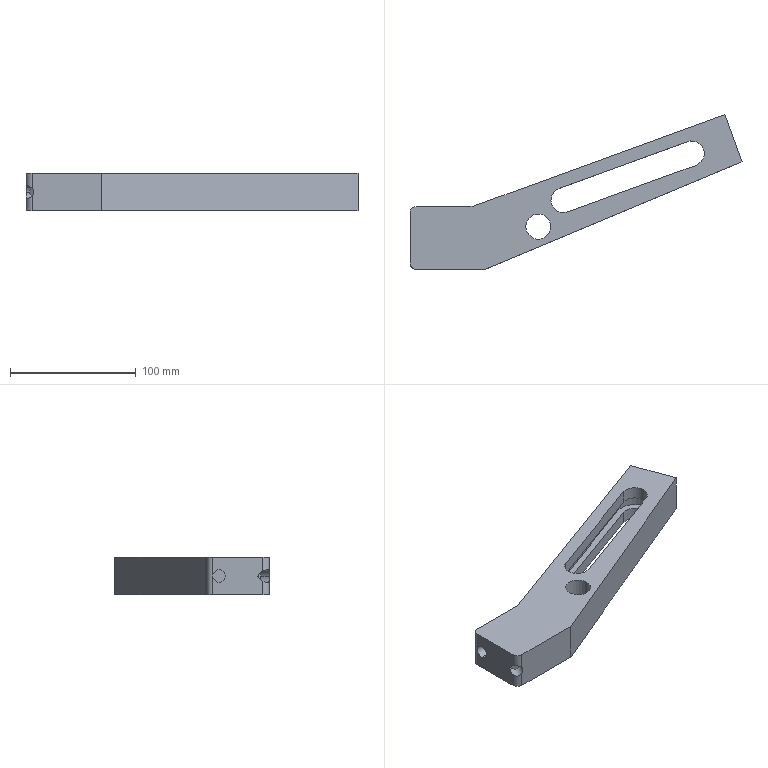Part | SolidWorks | features ICE 8, Fillet 2, Extrusion 1 | 1 solid | 37 faces | box 264.316 x 123.025 x 30 mm | volume 276042 mm3 | cylinder 19 | plane 18 | commonest cylinder face diameters 20 x9 10 x7 30 x3
STEP:
#1=CARTESIAN_POINT('',(239.287,92.152,-5.));
#2=VERTEX_POINT('',#1);
#3=CARTESIAN_POINT('',(219.156,106.247,-5.));
#4=VERTEX_POINT('',#3);
#5=CARTESIAN_POINT('',(224.287,92.152,-5.));
#6=DIRECTION('',(0.,0.,1.));
#7=DIRECTION('',(1.,0.,0.));
#8=AXIS2_PLACEMENT_3D('',#5,#6,#7);
#9=CIRCLE('',#8,15.);
#10=EDGE_CURVE('',#2,#4,#9,.T.);
#11=ORIENTED_EDGE('',*,*,#10,.F.);
#12=CARTESIAN_POINT('',(239.287,92.152,5.));
#13=VERTEX_POINT('',#12);
#14=CARTESIAN_POINT('',(239.287,92.152,-5.));
#15=DIRECTION('',(0.,0.,1.));
#16=VECTOR('',#15,1000.);
#17=LINE('',#14,#16);
#18=EDGE_CURVE('',#2,#13,#17,.T.);
#19=ORIENTED_EDGE('',*,*,#18,.T.);
#20=CARTESIAN_POINT('',(219.156,106.247,5.));
#21=VERTEX_POINT('',#20);
#22=CARTESIAN_POINT('',(224.287,92.152,5.));
#23=DIRECTION('',(0.,0.,1.));
#24=DIRECTION('',(1.,0.,0.));
#25=AXIS2_PLACEMENT_3D('',#22,#23,#24);
#26=CIRCLE('',#25,15.);
#27=EDGE_CURVE('',#13,#21,#26,.T.);
#28=ORIENTED_EDGE('',*,*,#27,.T.);
#29=CARTESIAN_POINT('',(219.156,106.247,-5.));
#30=DIRECTION('',(0.,0.,1.));
#31=VECTOR('',#30,1000.);
#32=LINE('',#29,#31);
#33=EDGE_CURVE('',#4,#21,#32,.T.);
#34=ORIENTED_EDGE('',*,*,#33,.F.);
#35=EDGE_LOOP('',(#11,#19,#28,#34));
#36=FACE_OUTER_BOUND('',#35,.T.);
#37=CARTESIAN_POINT('',(224.287,92.152,-5.));
#38=DIRECTION('',(0.,0.,1.));
#39=DIRECTION('',(1.,0.,0.));
#40=AXIS2_PLACEMENT_3D('',#37,#38,#39);
#41=CYLINDRICAL_SURFACE('',#40,15.);
#42=ADVANCED_FACE('',(#36),#41,.F.);
#43=CARTESIAN_POINT('',(112.167,33.891,-15.));
#44=VERTEX_POINT('',#43);
#45=CARTESIAN_POINT('',(92.167,33.891,-15.));
#46=VERTEX_POINT('',#45);
#47=CARTESIAN_POINT('',(102.167,33.891,-15.));
#48=DIRECTION('',(0.,0.,-1.));
#49=DIRECTION('',(-1.,0.,0.));
#50=AXIS2_PLACEMENT_3D('',#47,#48,#49);
#51=CIRCLE('',#50,10.);
#52=EDGE_CURVE('',#44,#46,#51,.T.);
#53=ORIENTED_EDGE('',*,*,#52,.T.);
#54=CARTESIAN_POINT('',(92.167,33.891,15.));
#55=VERTEX_POINT('',#54);
#56=CARTESIAN_POINT('',(92.167,33.891,-65.));
#57=DIRECTION('',(0.,0.,1.));
#58=VECTOR('',#57,1000.);
#59=LINE('',#56,#58);
#60=EDGE_CURVE('',#46,#55,#59,.T.);
#61=ORIENTED_EDGE('',*,*,#60,.T.);
#62=CARTESIAN_POINT('',(112.167,33.891,15.));
#63=VERTEX_POINT('',#62);
#64=CARTESIAN_POINT('',(102.167,33.891,15.));
#65=DIRECTION('',(0.,0.,1.));
#66=DIRECTION('',(1.,0.,0.));
#67=AXIS2_PLACEMENT_3D('',#64,#65,#66);
#68=CIRCLE('',#67,10.);
#69=EDGE_CURVE('',#55,#63,#68,.T.);
#70=ORIENTED_EDGE('',*,*,#69,.T.);
#71=CARTESIAN_POINT('',(112.167,33.891,-65.));
#72=DIRECTION('',(0.,0.,1.));
#73=VECTOR('',#72,1000.);
#74=LINE('',#71,#73);
#75=EDGE_CURVE('',#44,#63,#74,.T.);
#76=ORIENTED_EDGE('',*,*,#75,.F.);
#77=EDGE_LOOP('',(#53,#61,#70,#76));
#78=FACE_OUTER_BOUND('',#77,.T.);
#79=CARTESIAN_POINT('',(102.167,33.891,-65.));
#80=DIRECTION('',(0.,0.,1.));
#81=DIRECTION('',(1.,0.,0.));
#82=AXIS2_PLACEMENT_3D('',#79,#80,#81);
#83=CYLINDRICAL_SURFACE('',#82,10.);
#84=ADVANCED_FACE('',(#78),#83,.F.);
#85=CARTESIAN_POINT('',(10.,40.,-5.));
#86=VERTEX_POINT('',#85);
#87=CARTESIAN_POINT('',(10.,40.,5.));
#88=VERTEX_POINT('',#87);
#89=CARTESIAN_POINT('',(10.,40.,0.));
#90=DIRECTION('',(-1.,0.,0.));
#91=DIRECTION('',(0.,0.,1.));
#92=AXIS2_PLACEMENT_3D('',#89,#90,#91);
#93=CIRCLE('',#92,5.);
#94=EDGE_CURVE('',#86,#88,#93,.T.);
#95=ORIENTED_EDGE('',*,*,#94,.F.);
#96=CARTESIAN_POINT('',(0.,40.,-5.));
#97=VERTEX_POINT('',#96);
#98=CARTESIAN_POINT('',(10.,40.,-5.));
#99=DIRECTION('',(-1.,0.,0.));
#100=VECTOR('',#99,1000.);
#101=LINE('',#98,#100);
#102=EDGE_CURVE('',#86,#97,#101,.T.);
#103=ORIENTED_EDGE('',*,*,#102,.T.);
#104=CARTESIAN_POINT('',(0.,40.,5.));
#105=VERTEX_POINT('',#104);
#106=CARTESIAN_POINT('',(0.,40.,0.));
#107=DIRECTION('',(-1.,0.,0.));
#108=DIRECTION('',(0.,0.,1.));
#109=AXIS2_PLACEMENT_3D('',#106,#107,#108);
#110=CIRCLE('',#109,5.);
#111=EDGE_CURVE('',#97,#105,#110,.T.);
#112=ORIENTED_EDGE('',*,*,#111,.T.);
#113=CARTESIAN_POINT('',(10.,40.,5.));
#114=DIRECTION('',(-1.,0.,0.));
#115=VECTOR('',#114,1000.);
#116=LINE('',#113,#115);
#117=EDGE_CURVE('',#88,#105,#116,.T.);
#118=ORIENTED_EDGE('',*,*,#117,.F.);
#119=EDGE_LOOP('',(#95,#103,#112,#118));
#120=FACE_OUTER_BOUND('',#119,.T.);
#121=CARTESIAN_POINT('',(10.,40.,0.));
#122=DIRECTION('',(-1.,0.,0.));
#123=DIRECTION('',(0.,0.,1.));
#124=AXIS2_PLACEMENT_3D('',#121,#122,#123);
#125=CYLINDRICAL_SURFACE('',#124,5.);
#126=ADVANCED_FACE('',(#120),#125,.F.);
#127=CARTESIAN_POINT('',(2.999,12.634,0.));
#128=VERTEX_POINT('',#127);
#129=CARTESIAN_POINT('',(11.089,6.756,0.));
#130=VERTEX_POINT('',#129);
#131=CARTESIAN_POINT('',(7.044,9.695,0.));
#132=DIRECTION('',(-0.5878,-0.809,0.));
#133=DIRECTION('',(0.809,-0.5878,0.));
#134=AXIS2_PLACEMENT_3D('',#131,#132,#133);
#135=CIRCLE('',#134,5.);
#136=EDGE_CURVE('',#128,#130,#135,.T.);
#137=ORIENTED_EDGE('',*,*,#136,.F.);
#138=CARTESIAN_POINT('',(0.,8.507,0.));
#139=VERTEX_POINT('',#138);
#140=CARTESIAN_POINT('',(2.999,12.634,0.));
#141=DIRECTION('',(-0.5878,-0.809,0.));
#142=VECTOR('',#141,1000.);
#143=LINE('',#140,#142);
#144=EDGE_CURVE('',#128,#139,#143,.T.);
#145=ORIENTED_EDGE('',*,*,#144,.T.);
#146=CARTESIAN_POINT('',(0.,5.,-4.045));
#147=VERTEX_POINT('',#146);
#148=CARTESIAN_POINT('',(0.,5.,-4.045));
#149=CARTESIAN_POINT('',(0.,7.246,-3.086));
#150=CARTESIAN_POINT('',(0.,8.507,-1.632));
#151=CARTESIAN_POINT('',(0.,8.507,0.));
#152=(BOUNDED_CURVE()B_SPLINE_CURVE(3,(#148,#149,#150,#151),.UNSPECIFIED.,.F.,.T.)B_SPLINE_CURVE_WITH_KNOTS((4,4),(2.199,3.142),.UNSPECIFIED.)CURVE()GEOMETRIC_REPRESENTATION_ITEM()RATIONAL_B_SPLINE_CURVE((1.,0.9273,0.9273,1.))REPRESENTATION_ITEM(''));
#153=EDGE_CURVE('',#147,#139,#152,.T.);
#154=ORIENTED_EDGE('',*,*,#153,.F.);
#155=CARTESIAN_POINT('',(5.,0.,-2.939));
#156=VERTEX_POINT('',#155);
#157=CARTESIAN_POINT('',(0.,5.,-4.045));
#158=CARTESIAN_POINT('',(0.,4.668,-4.187));
#159=CARTESIAN_POINT('',(0.03262,4.339,-4.325));
#160=CARTESIAN_POINT('',(0.165,3.683,-4.577));
#161=CARTESIAN_POINT('',(0.2668,3.352,-4.692));
#162=CARTESIAN_POINT('',(0.4713,2.874,-4.828));
#163=CARTESIAN_POINT('',(0.5481,2.717,-4.868));
#164=CARTESIAN_POINT('',(0.7198,2.409,-4.933));
#165=CARTESIAN_POINT('',(0.8156,2.257,-4.958));
#166=CARTESIAN_POINT('',(1.127,1.817,-5.009));
#167=CARTESIAN_POINT('',(1.363,1.55,-5.009));
#168=CARTESIAN_POINT('',(1.758,1.189,-4.951));
#169=CARTESIAN_POINT('',(1.898,1.075,-4.921));
#170=CARTESIAN_POINT('',(2.181,0.8669,-4.843));
#171=CARTESIAN_POINT('',(2.325,0.7723,-4.795));
#172=CARTESIAN_POINT('',(2.619,0.6003,-4.681));
#173=CARTESIAN_POINT('',(2.769,0.5224,-4.615));
#174=CARTESIAN_POINT('',(3.068,0.3854,-4.466));
#175=CARTESIAN_POINT('',(3.217,0.3263,-4.384));
#176=CARTESIAN_POINT('',(3.659,0.1732,-4.117));
#177=CARTESIAN_POINT('',(3.951,0.1035,-3.909));
#178=CARTESIAN_POINT('',(4.499,0.01743,-3.455));
#179=CARTESIAN_POINT('',(4.758,0.,-3.208));
#180=CARTESIAN_POINT('',(5.,0.,-2.939));
#181=B_SPLINE_CURVE_WITH_KNOTS('',3,(#157,#158,#159,#160,#161,#162,#163,#164,#165,#166,#167,#168,#169,#170,#171,#172,#173,#174,#175,#176,#177,#178,#179,#180),.UNSPECIFIED.,.F.,.F.,(4,2,2,2,2,2,2,2,2,2,2,4),(0.,0.001072,0.002144,0.00268,0.003216,0.004288,0.004824,0.00536,0.005896,0.006432,0.007504,0.008576),.UNSPECIFIED.);
#182=EDGE_CURVE('',#147,#156,#181,.T.);
#183=ORIENTED_EDGE('',*,*,#182,.T.);
#184=CARTESIAN_POINT('',(6.18,0.,0.));
#185=VERTEX_POINT('',#184);
#186=CARTESIAN_POINT('',(6.18,0.,0.));
#187=CARTESIAN_POINT('',(6.18,0.,-1.065));
#188=CARTESIAN_POINT('',(5.774,0.,-2.077));
#189=CARTESIAN_POINT('',(5.,0.,-2.939));
#190=(BOUNDED_CURVE()B_SPLINE_CURVE(3,(#186,#187,#188,#189),.UNSPECIFIED.,.F.,.F.)B_SPLINE_CURVE_WITH_KNOTS((4,4),(3.142,3.77),.UNSPECIFIED.)CURVE()GEOMETRIC_REPRESENTATION_ITEM()RATIONAL_B_SPLINE_CURVE((1.,0.9674,0.9674,1.))REPRESENTATION_ITEM(''));
#191=EDGE_CURVE('',#185,#156,#190,.T.);
#192=ORIENTED_EDGE('',*,*,#191,.F.);
#193=CARTESIAN_POINT('',(11.089,6.756,0.));
#194=DIRECTION('',(-0.5878,-0.809,0.));
#195=VECTOR('',#194,1000.);
#196=LINE('',#193,#195);
#197=EDGE_CURVE('',#130,#185,#196,.T.);
#198=ORIENTED_EDGE('',*,*,#197,.F.);
#199=EDGE_LOOP('',(#137,#145,#154,#183,#192,#198));
#200=FACE_OUTER_BOUND('',#199,.T.);
#201=CARTESIAN_POINT('',(7.044,9.695,0.));
#202=DIRECTION('',(-0.5878,-0.809,0.));
#203=DIRECTION('',(0.809,-0.5878,0.));
#204=AXIS2_PLACEMENT_3D('',#201,#202,#203);
#205=CYLINDRICAL_SURFACE('',#204,5.);
#206=ADVANCED_FACE('',(#200),#205,.F.);
#207=CARTESIAN_POINT('',(118.809,64.403,15.));
#208=VERTEX_POINT('',#207);
#209=CARTESIAN_POINT('',(112.229,55.006,15.));
#210=VERTEX_POINT('',#209);
#211=CARTESIAN_POINT('',(122.229,55.006,15.));
#212=DIRECTION('',(0.,0.,1.));
#213=DIRECTION('',(1.,0.,0.));
#214=AXIS2_PLACEMENT_3D('',#211,#212,#213);
#215=CIRCLE('',#214,10.);
#216=EDGE_CURVE('',#208,#210,#215,.T.);
#217=ORIENTED_EDGE('',*,*,#216,.T.);
#218=CARTESIAN_POINT('',(112.229,55.006,5.));
#219=VERTEX_POINT('',#218);
#220=CARTESIAN_POINT('',(112.229,55.006,15.));
#221=DIRECTION('',(0.,0.,-1.));
#222=VECTOR('',#221,1000.);
#223=LINE('',#220,#222);
#224=EDGE_CURVE('',#210,#219,#223,.T.);
#225=ORIENTED_EDGE('',*,*,#224,.T.);
#226=CARTESIAN_POINT('',(118.809,64.403,5.));
#227=VERTEX_POINT('',#226);
#228=CARTESIAN_POINT('',(122.229,55.006,5.));
#229=DIRECTION('',(0.,0.,1.));
#230=DIRECTION('',(1.,0.,0.));
#231=AXIS2_PLACEMENT_3D('',#228,#229,#230);
#232=CIRCLE('',#231,10.);
#233=EDGE_CURVE('',#227,#219,#232,.T.);
#234=ORIENTED_EDGE('',*,*,#233,.F.);
#235=CARTESIAN_POINT('',(118.809,64.403,15.));
#236=DIRECTION('',(0.,0.,-1.));
#237=VECTOR('',#236,1000.);
#238=LINE('',#235,#237);
#239=EDGE_CURVE('',#208,#227,#238,.T.);
#240=ORIENTED_EDGE('',*,*,#239,.F.);
#241=EDGE_LOOP('',(#217,#225,#234,#240));
#242=FACE_OUTER_BOUND('',#241,.T.);
#243=CARTESIAN_POINT('',(122.229,55.006,15.));
#244=DIRECTION('',(0.,0.,-1.));
#245=DIRECTION('',(-1.,0.,0.));
#246=AXIS2_PLACEMENT_3D('',#243,#244,#245);
#247=CYLINDRICAL_SURFACE('',#246,10.);
#248=ADVANCED_FACE('',(#242),#247,.F.);
#249=CARTESIAN_POINT('',(118.809,64.403,-5.));
#250=VERTEX_POINT('',#249);
#251=CARTESIAN_POINT('',(112.229,55.006,-5.));
#252=VERTEX_POINT('',#251);
#253=CARTESIAN_POINT('',(122.229,55.006,-5.));
#254=DIRECTION('',(0.,0.,1.));
#255=DIRECTION('',(1.,0.,0.));
#256=AXIS2_PLACEMENT_3D('',#253,#254,#255);
#257=CIRCLE('',#256,10.);
#258=EDGE_CURVE('',#250,#252,#257,.T.);
#259=ORIENTED_EDGE('',*,*,#258,.T.);
#260=CARTESIAN_POINT('',(112.229,55.006,-15.));
#261=VERTEX_POINT('',#260);
#262=CARTESIAN_POINT('',(112.229,55.006,15.));
#263=DIRECTION('',(0.,0.,-1.));
#264=VECTOR('',#263,1000.);
#265=LINE('',#262,#264);
#266=EDGE_CURVE('',#252,#261,#265,.T.);
#267=ORIENTED_EDGE('',*,*,#266,.T.);
#268=CARTESIAN_POINT('',(118.809,64.403,-15.));
#269=VERTEX_POINT('',#268);
#270=CARTESIAN_POINT('',(122.229,55.006,-15.));
#271=DIRECTION('',(0.,0.,1.));
#272=DIRECTION('',(1.,0.,0.));
#273=AXIS2_PLACEMENT_3D('',#270,#271,#272);
#274=CIRCLE('',#273,10.);
#275=EDGE_CURVE('',#269,#261,#274,.T.);
#276=ORIENTED_EDGE('',*,*,#275,.F.);
#277=CARTESIAN_POINT('',(118.809,64.403,15.));
#278=DIRECTION('',(0.,0.,-1.));
#279=VECTOR('',#278,1000.);
#280=LINE('',#277,#279);
#281=EDGE_CURVE('',#250,#269,#280,.T.);
#282=ORIENTED_EDGE('',*,*,#281,.F.);
#283=EDGE_LOOP('',(#259,#267,#276,#282));
#284=FACE_OUTER_BOUND('',#283,.T.);
#285=CARTESIAN_POINT('',(122.229,55.006,15.));
#286=DIRECTION('',(0.,0.,-1.));
#287=DIRECTION('',(-1.,0.,0.));
#288=AXIS2_PLACEMENT_3D('',#285,#286,#287);
#289=CYLINDRICAL_SURFACE('',#288,10.);
#290=ADVANCED_FACE('',(#284),#289,.F.);
#291=ORIENTED_EDGE('',*,*,#266,.F.);
#292=CARTESIAN_POINT('',(125.649,45.609,-5.));
#293=VERTEX_POINT('',#292);
#294=CARTESIAN_POINT('',(122.229,55.006,-5.));
#295=DIRECTION('',(0.,0.,1.));
#296=DIRECTION('',(1.,0.,0.));
#297=AXIS2_PLACEMENT_3D('',#294,#295,#296);
#298=CIRCLE('',#297,10.);
#299=EDGE_CURVE('',#252,#293,#298,.T.);
#300=ORIENTED_EDGE('',*,*,#299,.T.);
#301=CARTESIAN_POINT('',(125.649,45.609,-15.));
#302=VERTEX_POINT('',#301);
#303=CARTESIAN_POINT('',(125.649,45.609,15.));
#304=DIRECTION('',(0.,0.,-1.));
#305=VECTOR('',#304,1000.);
#306=LINE('',#303,#305);
#307=EDGE_CURVE('',#293,#302,#306,.T.);
#308=ORIENTED_EDGE('',*,*,#307,.T.);
#309=CARTESIAN_POINT('',(122.229,55.006,-15.));
#310=DIRECTION('',(0.,0.,1.));
#311=DIRECTION('',(1.,0.,0.));
#312=AXIS2_PLACEMENT_3D('',#309,#310,#311);
#313=CIRCLE('',#312,10.);
#314=EDGE_CURVE('',#261,#302,#313,.T.);
#315=ORIENTED_EDGE('',*,*,#314,.F.);
#316=EDGE_LOOP('',(#291,#300,#308,#315));
#317=FACE_OUTER_BOUND('',#316,.T.);
#318=CARTESIAN_POINT('',(122.229,55.006,15.));
#319=DIRECTION('',(0.,0.,-1.));
#320=DIRECTION('',(-1.,0.,0.));
#321=AXIS2_PLACEMENT_3D('',#318,#319,#320);
#322=CYLINDRICAL_SURFACE('',#321,10.);
#323=ADVANCED_FACE('',(#317),#322,.F.);
#324=ORIENTED_EDGE('',*,*,#307,.F.);
#325=CARTESIAN_POINT('',(227.707,82.755,-5.));
#326=VERTEX_POINT('',#325);
#327=CARTESIAN_POINT('',(125.649,45.609,-5.));
#328=DIRECTION('',(0.9397,0.342,0.));
#329=VECTOR('',#328,1000.);
#330=LINE('',#327,#329);
#331=EDGE_CURVE('',#293,#326,#330,.T.);
#332=ORIENTED_EDGE('',*,*,#331,.T.);
#333=CARTESIAN_POINT('',(227.707,82.755,-15.));
#334=VERTEX_POINT('',#333);
#335=CARTESIAN_POINT('',(227.707,82.755,15.));
#336=DIRECTION('',(0.,0.,-1.));
#337=VECTOR('',#336,1000.);
#338=LINE('',#335,#337);
#339=EDGE_CURVE('',#326,#334,#338,.T.);
#340=ORIENTED_EDGE('',*,*,#339,.T.);
#341=CARTESIAN_POINT('',(125.649,45.609,-15.));
#342=DIRECTION('',(0.9397,0.342,0.));
#343=VECTOR('',#342,1000.);
#344=LINE('',#341,#343);
#345=EDGE_CURVE('',#302,#334,#344,.T.);
#346=ORIENTED_EDGE('',*,*,#345,.F.);
#347=EDGE_LOOP('',(#324,#332,#340,#346));
#348=FACE_OUTER_BOUND('',#347,.T.);
#349=CARTESIAN_POINT('',(125.649,45.609,15.));
#350=DIRECTION('',(-0.342,0.9397,0.));
#351=DIRECTION('',(-0.9397,-0.342,0.));
#352=AXIS2_PLACEMENT_3D('',#349,#350,#351);
#353=PLANE('',#352);
#354=ADVANCED_FACE('',(#348),#353,.T.);
#355=ORIENTED_EDGE('',*,*,#339,.F.);
#356=CARTESIAN_POINT('',(220.867,101.549,-5.));
#357=VERTEX_POINT('',#356);
#358=CARTESIAN_POINT('',(224.287,92.152,-5.));
#359=DIRECTION('',(0.,0.,1.));
#360=DIRECTION('',(1.,0.,0.));
#361=AXIS2_PLACEMENT_3D('',#358,#359,#360);
#362=CIRCLE('',#361,10.);
#363=EDGE_CURVE('',#326,#357,#362,.T.);
#364=ORIENTED_EDGE('',*,*,#363,.T.);
#365=CARTESIAN_POINT('',(220.867,101.549,-15.));
#366=VERTEX_POINT('',#365);
#367=CARTESIAN_POINT('',(220.867,101.549,15.));
#368=DIRECTION('',(0.,0.,-1.));
#369=VECTOR('',#368,1000.);
#370=LINE('',#367,#369);
#371=EDGE_CURVE('',#357,#366,#370,.T.);
#372=ORIENTED_EDGE('',*,*,#371,.T.);
#373=CARTESIAN_POINT('',(224.287,92.152,-15.));
#374=DIRECTION('',(0.,0.,1.));
#375=DIRECTION('',(1.,0.,0.));
#376=AXIS2_PLACEMENT_3D('',#373,#374,#375);
#377=CIRCLE('',#376,10.);
#378=EDGE_CURVE('',#334,#366,#377,.T.);
#379=ORIENTED_EDGE('',*,*,#378,.F.);
#380=EDGE_LOOP('',(#355,#364,#372,#379));
#381=FACE_OUTER_BOUND('',#380,.T.);
#382=CARTESIAN_POINT('',(224.287,92.152,15.));
#383=DIRECTION('',(0.,0.,-1.));
#384=DIRECTION('',(-1.,0.,0.));
#385=AXIS2_PLACEMENT_3D('',#382,#383,#384);
#386=CYLINDRICAL_SURFACE('',#385,10.);
#387=ADVANCED_FACE('',(#381),#386,.F.);
#388=ORIENTED_EDGE('',*,*,#371,.F.);
#389=CARTESIAN_POINT('',(220.867,101.549,-5.));
#390=DIRECTION('',(-0.9397,-0.342,0.));
#391=VECTOR('',#390,1000.);
#392=LINE('',#389,#391);
#393=EDGE_CURVE('',#357,#250,#392,.T.);
#394=ORIENTED_EDGE('',*,*,#393,.T.);
#395=ORIENTED_EDGE('',*,*,#281,.T.);
#396=CARTESIAN_POINT('',(118.809,64.403,-15.));
#397=DIRECTION('',(-0.9397,-0.342,0.));
#398=VECTOR('',#397,1000.);
#399=LINE('',#396,#398);
#400=EDGE_CURVE('',#366,#269,#399,.T.);
#401=ORIENTED_EDGE('',*,*,#400,.F.);
#402=EDGE_LOOP('',(#388,#394,#395,#401));
#403=FACE_OUTER_BOUND('',#402,.T.);
#404=CARTESIAN_POINT('',(118.809,64.403,15.));
#405=DIRECTION('',(0.342,-0.9397,0.));
#406=DIRECTION('',(0.9397,0.342,0.));
#407=AXIS2_PLACEMENT_3D('',#404,#405,#406);
#408=PLANE('',#407);
#409=ADVANCED_FACE('',(#403),#408,.T.);
#410=CARTESIAN_POINT('',(5.,0.,2.939));
#411=VERTEX_POINT('',#410);
#412=CARTESIAN_POINT('',(0.,5.,4.045));
#413=VERTEX_POINT('',#412);
#414=CARTESIAN_POINT('',(5.,0.,2.939));
#415=CARTESIAN_POINT('',(4.758,0.,3.208));
#416=CARTESIAN_POINT('',(4.5,0.0174,3.455));
#417=CARTESIAN_POINT('',(3.953,0.103,3.908));
#418=CARTESIAN_POINT('',(3.661,0.1726,4.116));
#419=CARTESIAN_POINT('',(3.22,0.325,4.382));
#420=CARTESIAN_POINT('',(3.072,0.3837,4.464));
#421=CARTESIAN_POINT('',(2.775,0.5192,4.612));
#422=CARTESIAN_POINT('',(2.625,0.5967,4.679));
#423=CARTESIAN_POINT('',(2.182,0.8555,4.851));
#424=CARTESIAN_POINT('',(1.901,1.06,4.929));
#425=CARTESIAN_POINT('',(1.505,1.42,4.989));
#426=CARTESIAN_POINT('',(1.376,1.55,4.999));
#427=CARTESIAN_POINT('',(1.138,1.819,5.001));
#428=CARTESIAN_POINT('',(1.027,1.959,4.993));
#429=CARTESIAN_POINT('',(0.82,2.251,4.959));
#430=CARTESIAN_POINT('',(0.7237,2.403,4.934));
#431=CARTESIAN_POINT('',(0.5503,2.713,4.869));
#432=CARTESIAN_POINT('',(0.473,2.87,4.829));
#433=CARTESIAN_POINT('',(0.2677,3.349,4.693));
#434=CARTESIAN_POINT('',(0.1657,3.68,4.578));
#435=CARTESIAN_POINT('',(0.03268,4.338,4.325));
#436=CARTESIAN_POINT('',(0.,4.667,4.187));
#437=CARTESIAN_POINT('',(0.,5.,4.045));
#438=B_SPLINE_CURVE_WITH_KNOTS('',3,(#414,#415,#416,#417,#418,#419,#420,#421,#422,#423,#424,#425,#426,#427,#428,#429,#430,#431,#432,#433,#434,#435,#436,#437),.UNSPECIFIED.,.F.,.F.,(4,2,2,2,2,2,2,2,2,2,2,4),(0.,0.001072,0.002144,0.00268,0.003216,0.004288,0.004824,0.00536,0.005896,0.006432,0.007504,0.008576),.UNSPECIFIED.);
#439=EDGE_CURVE('',#411,#413,#438,.T.);
#440=ORIENTED_EDGE('',*,*,#439,.F.);
#441=CARTESIAN_POINT('',(5.,0.,15.));
#442=VERTEX_POINT('',#441);
#443=CARTESIAN_POINT('',(5.,0.,15.));
#444=DIRECTION('',(0.,0.,-1.));
#445=VECTOR('',#444,1000.);
#446=LINE('',#443,#445);
#447=EDGE_CURVE('',#442,#411,#446,.T.);
#448=ORIENTED_EDGE('',*,*,#447,.F.);
#449=CARTESIAN_POINT('',(0.,5.,15.));
#450=VERTEX_POINT('',#449);
#451=CARTESIAN_POINT('',(5.,5.,15.));
#452=DIRECTION('',(0.,0.,1.));
#453=DIRECTION('',(-1.,0.,0.));
#454=AXIS2_PLACEMENT_3D('',#451,#452,#453);
#455=CIRCLE('',#454,5.);
#456=EDGE_CURVE('',#450,#442,#455,.T.);
#457=ORIENTED_EDGE('',*,*,#456,.F.);
#458=CARTESIAN_POINT('',(0.,5.,15.));
#459=DIRECTION('',(0.,0.,1.));
#460=VECTOR('',#459,1000.);
#461=LINE('',#458,#460);
#462=EDGE_CURVE('',#413,#450,#461,.T.);
#463=ORIENTED_EDGE('',*,*,#462,.F.);
#464=EDGE_LOOP('',(#440,#448,#457,#463));
#465=FACE_OUTER_BOUND('',#464,.T.);
#466=CARTESIAN_POINT('',(5.,5.,15.));
#467=DIRECTION('',(0.,0.,-1.));
#468=DIRECTION('',(-1.,0.,0.));
#469=AXIS2_PLACEMENT_3D('',#466,#467,#468);
#470=CYLINDRICAL_SURFACE('',#469,5.);
#471=ADVANCED_FACE('',(#465),#470,.T.);
#472=CARTESIAN_POINT('',(102.167,33.891,15.));
#473=DIRECTION('',(0.,0.,1.));
#474=DIRECTION('',(1.,0.,0.));
#475=AXIS2_PLACEMENT_3D('',#472,#473,#474);
#476=CIRCLE('',#475,10.);
#477=EDGE_CURVE('',#63,#55,#476,.T.);
#478=ORIENTED_EDGE('',*,*,#477,.F.);
#479=ORIENTED_EDGE('',*,*,#69,.F.);
#480=EDGE_LOOP('',(#478,#479));
#481=FACE_BOUND('',#480,.T.);
#482=CARTESIAN_POINT('',(0.,45.,15.));
#483=VERTEX_POINT('',#482);
#484=CARTESIAN_POINT('',(0.,0.,15.));
#485=DIRECTION('',(0.,-1.,0.));
#486=VECTOR('',#485,1000.);
#487=LINE('',#484,#486);
#488=EDGE_CURVE('',#483,#450,#487,.T.);
#489=ORIENTED_EDGE('',*,*,#488,.T.);
#490=ORIENTED_EDGE('',*,*,#456,.T.);
#491=CARTESIAN_POINT('',(60.,0.,15.));
#492=VERTEX_POINT('',#491);
#493=CARTESIAN_POINT('',(60.,0.,15.));
#494=DIRECTION('',(1.,0.,0.));
#495=VECTOR('',#494,1000.);
#496=LINE('',#493,#495);
#497=EDGE_CURVE('',#442,#492,#496,.T.);
#498=ORIENTED_EDGE('',*,*,#497,.T.);
#499=CARTESIAN_POINT('',(264.316,85.437,15.));
#500=VERTEX_POINT('',#499);
#501=CARTESIAN_POINT('',(264.316,85.437,15.));
#502=DIRECTION('',(0.9226,0.3858,0.));
#503=VECTOR('',#502,1000.);
#504=LINE('',#501,#503);
#505=EDGE_CURVE('',#492,#500,#504,.T.);
#506=ORIENTED_EDGE('',*,*,#505,.T.);
#507=CARTESIAN_POINT('',(250.635,123.025,15.));
#508=VERTEX_POINT('',#507);
#509=CARTESIAN_POINT('',(250.635,123.025,15.));
#510=DIRECTION('',(-0.342,0.9397,0.));
#511=VECTOR('',#510,1000.);
#512=LINE('',#509,#511);
#513=EDGE_CURVE('',#500,#508,#512,.T.);
#514=ORIENTED_EDGE('',*,*,#513,.T.);
#515=CARTESIAN_POINT('',(51.657,50.603,15.));
#516=VERTEX_POINT('',#515);
#517=CARTESIAN_POINT('',(50.,50.,15.));
#518=DIRECTION('',(-0.9397,-0.342,0.));
#519=VECTOR('',#518,1000.);
#520=LINE('',#517,#519);
#521=EDGE_CURVE('',#508,#516,#520,.T.);
#522=ORIENTED_EDGE('',*,*,#521,.T.);
#523=CARTESIAN_POINT('',(48.237,50.,15.));
#524=VERTEX_POINT('',#523);
#525=CARTESIAN_POINT('',(48.237,60.,15.));
#526=DIRECTION('',(0.,0.,-1.));
#527=DIRECTION('',(-1.,0.,0.));
#528=AXIS2_PLACEMENT_3D('',#525,#526,#527);
#529=CIRCLE('',#528,10.);
#530=EDGE_CURVE('',#516,#524,#529,.T.);
#531=ORIENTED_EDGE('',*,*,#530,.T.);
#532=CARTESIAN_POINT('',(5.,50.,15.));
#533=VERTEX_POINT('',#532);
#534=CARTESIAN_POINT('',(0.,50.,15.));
#535=DIRECTION('',(-1.,0.,0.));
#536=VECTOR('',#535,1000.);
#537=LINE('',#534,#536);
#538=EDGE_CURVE('',#524,#533,#537,.T.);
#539=ORIENTED_EDGE('',*,*,#538,.T.);
#540=CARTESIAN_POINT('',(5.,45.,15.));
#541=DIRECTION('',(0.,0.,1.));
#542=DIRECTION('',(-1.,0.,0.));
#543=AXIS2_PLACEMENT_3D('',#540,#541,#542);
#544=CIRCLE('',#543,5.);
#545=EDGE_CURVE('',#533,#483,#544,.T.);
#546=ORIENTED_EDGE('',*,*,#545,.T.);
#547=EDGE_LOOP('',(#489,#490,#498,#506,#514,#522,#531,#539,#546));
#548=FACE_OUTER_BOUND('',#547,.T.);
#549=ORIENTED_EDGE('',*,*,#216,.F.);
#550=CARTESIAN_POINT('',(220.867,101.549,15.));
#551=VERTEX_POINT('',#550);
#552=CARTESIAN_POINT('',(118.809,64.403,15.));
#553=DIRECTION('',(-0.9397,-0.342,0.));
#554=VECTOR('',#553,1000.);
#555=LINE('',#552,#554);
#556=EDGE_CURVE('',#551,#208,#555,.T.);
#557=ORIENTED_EDGE('',*,*,#556,.F.);
#558=CARTESIAN_POINT('',(227.707,82.755,15.));
#559=VERTEX_POINT('',#558);
#560=CARTESIAN_POINT('',(224.287,92.152,15.));
#561=DIRECTION('',(0.,0.,1.));
#562=DIRECTION('',(1.,0.,0.));
#563=AXIS2_PLACEMENT_3D('',#560,#561,#562);
#564=CIRCLE('',#563,10.);
#565=EDGE_CURVE('',#559,#551,#564,.T.);
#566=ORIENTED_EDGE('',*,*,#565,.F.);
#567=CARTESIAN_POINT('',(125.649,45.609,15.));
#568=VERTEX_POINT('',#567);
#569=CARTESIAN_POINT('',(125.649,45.609,15.));
#570=DIRECTION('',(0.9397,0.342,0.));
#571=VECTOR('',#570,1000.);
#572=LINE('',#569,#571);
#573=EDGE_CURVE('',#568,#559,#572,.T.);
#574=ORIENTED_EDGE('',*,*,#573,.F.);
#575=CARTESIAN_POINT('',(122.229,55.006,15.));
#576=DIRECTION('',(0.,0.,1.));
#577=DIRECTION('',(1.,0.,0.));
#578=AXIS2_PLACEMENT_3D('',#575,#576,#577);
#579=CIRCLE('',#578,10.);
#580=EDGE_CURVE('',#210,#568,#579,.T.);
#581=ORIENTED_EDGE('',*,*,#580,.F.);
#582=EDGE_LOOP('',(#549,#557,#566,#574,#581));
#583=FACE_BOUND('',#582,.T.);
#584=CARTESIAN_POINT('',(0.,0.,15.));
#585=DIRECTION('',(0.,0.,-1.));
#586=DIRECTION('',(-1.,0.,0.));
#587=AXIS2_PLACEMENT_3D('',#584,#585,#586);
#588=PLANE('',#587);
#589=ADVANCED_FACE('',(#481,#548,#583),#588,.F.);
#590=CARTESIAN_POINT('',(48.237,50.,-15.));
#591=VERTEX_POINT('',#590);
#592=CARTESIAN_POINT('',(51.657,50.603,-15.));
#593=VERTEX_POINT('',#592);
#594=CARTESIAN_POINT('',(48.237,60.,-15.));
#595=DIRECTION('',(0.,0.,1.));
#596=DIRECTION('',(-1.,0.,0.));
#597=AXIS2_PLACEMENT_3D('',#594,#595,#596);
#598=CIRCLE('',#597,10.);
#599=EDGE_CURVE('',#591,#593,#598,.T.);
#600=ORIENTED_EDGE('',*,*,#599,.T.);
#601=CARTESIAN_POINT('',(250.635,123.025,-15.));
#602=VERTEX_POINT('',#601);
#603=CARTESIAN_POINT('',(50.,50.,-15.));
#604=DIRECTION('',(-0.9397,-0.342,0.));
#605=VECTOR('',#604,1000.);
#606=LINE('',#603,#605);
#607=EDGE_CURVE('',#602,#593,#606,.T.);
#608=ORIENTED_EDGE('',*,*,#607,.F.);
#609=CARTESIAN_POINT('',(264.316,85.437,-15.));
#610=VERTEX_POINT('',#609);
#611=CARTESIAN_POINT('',(250.635,123.025,-15.));
#612=DIRECTION('',(-0.342,0.9397,0.));
#613=VECTOR('',#612,1000.);
#614=LINE('',#611,#613);
#615=EDGE_CURVE('',#610,#602,#614,.T.);
#616=ORIENTED_EDGE('',*,*,#615,.F.);
#617=CARTESIAN_POINT('',(60.,0.,-15.));
#618=VERTEX_POINT('',#617);
#619=CARTESIAN_POINT('',(264.316,85.437,-15.));
#620=DIRECTION('',(0.9226,0.3858,0.));
#621=VECTOR('',#620,1000.);
#622=LINE('',#619,#621);
#623=EDGE_CURVE('',#618,#610,#622,.T.);
#624=ORIENTED_EDGE('',*,*,#623,.F.);
#625=CARTESIAN_POINT('',(5.,0.,-15.));
#626=VERTEX_POINT('',#625);
#627=CARTESIAN_POINT('',(60.,0.,-15.));
#628=DIRECTION('',(1.,0.,0.));
#629=VECTOR('',#628,1000.);
#630=LINE('',#627,#629);
#631=EDGE_CURVE('',#626,#618,#630,.T.);
#632=ORIENTED_EDGE('',*,*,#631,.F.);
#633=CARTESIAN_POINT('',(0.,5.,-15.));
#634=VERTEX_POINT('',#633);
#635=CARTESIAN_POINT('',(5.,5.,-15.));
#636=DIRECTION('',(0.,0.,-1.));
#637=DIRECTION('',(-1.,0.,0.));
#638=AXIS2_PLACEMENT_3D('',#635,#636,#637);
#639=CIRCLE('',#638,5.);
#640=EDGE_CURVE('',#626,#634,#639,.T.);
#641=ORIENTED_EDGE('',*,*,#640,.T.);
#642=CARTESIAN_POINT('',(0.,45.,-15.));
#643=VERTEX_POINT('',#642);
#644=CARTESIAN_POINT('',(0.,0.,-15.));
#645=DIRECTION('',(0.,-1.,0.));
#646=VECTOR('',#645,1000.);
#647=LINE('',#644,#646);
#648=EDGE_CURVE('',#643,#634,#647,.T.);
#649=ORIENTED_EDGE('',*,*,#648,.F.);
#650=CARTESIAN_POINT('',(5.,50.,-15.));
#651=VERTEX_POINT('',#650);
#652=CARTESIAN_POINT('',(5.,45.,-15.));
#653=DIRECTION('',(0.,0.,-1.));
#654=DIRECTION('',(-1.,0.,0.));
#655=AXIS2_PLACEMENT_3D('',#652,#653,#654);
#656=CIRCLE('',#655,5.);
#657=EDGE_CURVE('',#643,#651,#656,.T.);
#658=ORIENTED_EDGE('',*,*,#657,.T.);
#659=CARTESIAN_POINT('',(0.,50.,-15.));
#660=DIRECTION('',(-1.,0.,0.));
#661=VECTOR('',#660,1000.);
#662=LINE('',#659,#661);
#663=EDGE_CURVE('',#591,#651,#662,.T.);
#664=ORIENTED_EDGE('',*,*,#663,.F.);
#665=EDGE_LOOP('',(#600,#608,#616,#624,#632,#641,#649,#658,#664));
#666=FACE_OUTER_BOUND('',#665,.T.);
#667=ORIENTED_EDGE('',*,*,#400,.T.);
#668=ORIENTED_EDGE('',*,*,#275,.T.);
#669=ORIENTED_EDGE('',*,*,#314,.T.);
#670=ORIENTED_EDGE('',*,*,#345,.T.);
#671=ORIENTED_EDGE('',*,*,#378,.T.);
#672=EDGE_LOOP('',(#667,#668,#669,#670,#671));
#673=FACE_BOUND('',#672,.T.);
#674=ORIENTED_EDGE('',*,*,#52,.F.);
#675=CARTESIAN_POINT('',(102.167,33.891,-15.));
#676=DIRECTION('',(0.,0.,-1.));
#677=DIRECTION('',(-1.,0.,0.));
#678=AXIS2_PLACEMENT_3D('',#675,#676,#677);
#679=CIRCLE('',#678,10.);
#680=EDGE_CURVE('',#46,#44,#679,.T.);
#681=ORIENTED_EDGE('',*,*,#680,.F.);
#682=EDGE_LOOP('',(#674,#681));
#683=FACE_BOUND('',#682,.T.);
#684=CARTESIAN_POINT('',(0.,0.,-15.));
#685=DIRECTION('',(0.,0.,-1.));
#686=DIRECTION('',(-1.,0.,0.));
#687=AXIS2_PLACEMENT_3D('',#684,#685,#686);
#688=PLANE('',#687);
#689=ADVANCED_FACE('',(#666,#673,#683),#688,.T.);
#690=ORIENTED_EDGE('',*,*,#447,.T.);
#691=CARTESIAN_POINT('',(5.,0.,2.939));
#692=CARTESIAN_POINT('',(5.774,0.,2.077));
#693=CARTESIAN_POINT('',(6.18,0.,1.065));
#694=CARTESIAN_POINT('',(6.18,0.,0.));
#695=(BOUNDED_CURVE()B_SPLINE_CURVE(3,(#691,#692,#693,#694),.UNSPECIFIED.,.F.,.F.)B_SPLINE_CURVE_WITH_KNOTS((4,4),(2.513,3.142),.UNSPECIFIED.)CURVE()GEOMETRIC_REPRESENTATION_ITEM()RATIONAL_B_SPLINE_CURVE((1.,0.9674,0.9674,1.))REPRESENTATION_ITEM(''));
#696=EDGE_CURVE('',#411,#185,#695,.T.);
#697=ORIENTED_EDGE('',*,*,#696,.T.);
#698=ORIENTED_EDGE('',*,*,#191,.T.);
#699=CARTESIAN_POINT('',(5.,0.,15.));
#700=DIRECTION('',(0.,0.,-1.));
#701=VECTOR('',#700,1000.);
#702=LINE('',#699,#701);
#703=EDGE_CURVE('',#156,#626,#702,.T.);
#704=ORIENTED_EDGE('',*,*,#703,.T.);
#705=ORIENTED_EDGE('',*,*,#631,.T.);
#706=CARTESIAN_POINT('',(60.,0.,15.));
#707=DIRECTION('',(0.,0.,-1.));
#708=VECTOR('',#707,1000.);
#709=LINE('',#706,#708);
#710=EDGE_CURVE('',#492,#618,#709,.T.);
#711=ORIENTED_EDGE('',*,*,#710,.F.);
#712=ORIENTED_EDGE('',*,*,#497,.F.);
#713=EDGE_LOOP('',(#690,#697,#698,#704,#705,#711,#712));
#714=FACE_OUTER_BOUND('',#713,.T.);
#715=CARTESIAN_POINT('',(60.,0.,15.));
#716=DIRECTION('',(0.,1.,0.));
#717=DIRECTION('',(-1.,0.,0.));
#718=AXIS2_PLACEMENT_3D('',#715,#716,#717);
#719=PLANE('',#718);
#720=ADVANCED_FACE('',(#714),#719,.F.);
#721=ORIENTED_EDGE('',*,*,#623,.T.);
#722=CARTESIAN_POINT('',(264.316,85.437,15.));
#723=DIRECTION('',(0.,0.,-1.));
#724=VECTOR('',#723,1000.);
#725=LINE('',#722,#724);
#726=EDGE_CURVE('',#500,#610,#725,.T.);
#727=ORIENTED_EDGE('',*,*,#726,.F.);
#728=ORIENTED_EDGE('',*,*,#505,.F.);
#729=ORIENTED_EDGE('',*,*,#710,.T.);
#730=EDGE_LOOP('',(#721,#727,#728,#729));
#731=FACE_OUTER_BOUND('',#730,.T.);
#732=CARTESIAN_POINT('',(264.316,85.437,15.));
#733=DIRECTION('',(-0.3858,0.9226,0.));
#734=DIRECTION('',(-0.9226,-0.3858,0.));
#735=AXIS2_PLACEMENT_3D('',#732,#733,#734);
#736=PLANE('',#735);
#737=ADVANCED_FACE('',(#731),#736,.F.);
#738=ORIENTED_EDGE('',*,*,#615,.T.);
#739=CARTESIAN_POINT('',(250.635,123.025,15.));
#740=DIRECTION('',(0.,0.,-1.));
#741=VECTOR('',#740,1000.);
#742=LINE('',#739,#741);
#743=EDGE_CURVE('',#508,#602,#742,.T.);
#744=ORIENTED_EDGE('',*,*,#743,.F.);
#745=ORIENTED_EDGE('',*,*,#513,.F.);
#746=ORIENTED_EDGE('',*,*,#726,.T.);
#747=EDGE_LOOP('',(#738,#744,#745,#746));
#748=FACE_OUTER_BOUND('',#747,.T.);
#749=CARTESIAN_POINT('',(250.635,123.025,15.));
#750=DIRECTION('',(-0.9397,-0.342,0.));
#751=DIRECTION('',(0.342,-0.9397,0.));
#752=AXIS2_PLACEMENT_3D('',#749,#750,#751);
#753=PLANE('',#752);
#754=ADVANCED_FACE('',(#748),#753,.F.);
#755=ORIENTED_EDGE('',*,*,#607,.T.);
#756=CARTESIAN_POINT('',(51.657,50.603,15.));
#757=DIRECTION('',(0.,0.,1.));
#758=VECTOR('',#757,1000.);
#759=LINE('',#756,#758);
#760=EDGE_CURVE('',#593,#516,#759,.T.);
#761=ORIENTED_EDGE('',*,*,#760,.T.);
#762=ORIENTED_EDGE('',*,*,#521,.F.);
#763=ORIENTED_EDGE('',*,*,#743,.T.);
#764=EDGE_LOOP('',(#755,#761,#762,#763));
#765=FACE_OUTER_BOUND('',#764,.T.);
#766=CARTESIAN_POINT('',(50.,50.,15.));
#767=DIRECTION('',(0.342,-0.9397,0.));
#768=DIRECTION('',(0.9397,0.342,0.));
#769=AXIS2_PLACEMENT_3D('',#766,#767,#768);
#770=PLANE('',#769);
#771=ADVANCED_FACE('',(#765),#770,.F.);
#772=ORIENTED_EDGE('',*,*,#663,.T.);
#773=CARTESIAN_POINT('',(5.,50.,15.));
#774=DIRECTION('',(0.,0.,1.));
#775=VECTOR('',#774,1000.);
#776=LINE('',#773,#775);
#777=EDGE_CURVE('',#651,#533,#776,.T.);
#778=ORIENTED_EDGE('',*,*,#777,.T.);
#779=ORIENTED_EDGE('',*,*,#538,.F.);
#780=CARTESIAN_POINT('',(48.237,50.,-15.));
#781=DIRECTION('',(0.,0.,-1.));
#782=VECTOR('',#781,1000.);
#783=LINE('',#780,#782);
#784=EDGE_CURVE('',#524,#591,#783,.T.);
#785=ORIENTED_EDGE('',*,*,#784,.T.);
#786=EDGE_LOOP('',(#772,#778,#779,#785));
#787=FACE_OUTER_BOUND('',#786,.T.);
#788=CARTESIAN_POINT('',(0.,50.,15.));
#789=DIRECTION('',(0.,-1.,0.));
#790=DIRECTION('',(0.,0.,-1.));
#791=AXIS2_PLACEMENT_3D('',#788,#789,#790);
#792=PLANE('',#791);
#793=ADVANCED_FACE('',(#787),#792,.F.);
#794=CARTESIAN_POINT('',(0.,45.,0.));
#795=VERTEX_POINT('',#794);
#796=CARTESIAN_POINT('',(0.,45.,15.));
#797=DIRECTION('',(0.,0.,-1.));
#798=VECTOR('',#797,1000.);
#799=LINE('',#796,#798);
#800=EDGE_CURVE('',#483,#795,#799,.T.);
#801=ORIENTED_EDGE('',*,*,#800,.T.);
#802=CARTESIAN_POINT('',(0.,40.,0.));
#803=DIRECTION('',(-1.,0.,0.));
#804=DIRECTION('',(0.,0.,1.));
#805=AXIS2_PLACEMENT_3D('',#802,#803,#804);
#806=CIRCLE('',#805,5.);
#807=EDGE_CURVE('',#105,#795,#806,.T.);
#808=ORIENTED_EDGE('',*,*,#807,.F.);
#809=ORIENTED_EDGE('',*,*,#111,.F.);
#810=CARTESIAN_POINT('',(0.,40.,0.));
#811=DIRECTION('',(-1.,0.,0.));
#812=DIRECTION('',(0.,0.,1.));
#813=AXIS2_PLACEMENT_3D('',#810,#811,#812);
#814=CIRCLE('',#813,5.);
#815=EDGE_CURVE('',#795,#97,#814,.T.);
#816=ORIENTED_EDGE('',*,*,#815,.F.);
#817=CARTESIAN_POINT('',(0.,45.,15.));
#818=DIRECTION('',(0.,0.,-1.));
#819=VECTOR('',#818,1000.);
#820=LINE('',#817,#819);
#821=EDGE_CURVE('',#795,#643,#820,.T.);
#822=ORIENTED_EDGE('',*,*,#821,.T.);
#823=ORIENTED_EDGE('',*,*,#648,.T.);
#824=CARTESIAN_POINT('',(0.,5.,15.));
#825=DIRECTION('',(0.,0.,1.));
#826=VECTOR('',#825,1000.);
#827=LINE('',#824,#826);
#828=EDGE_CURVE('',#634,#147,#827,.T.);
#829=ORIENTED_EDGE('',*,*,#828,.T.);
#830=ORIENTED_EDGE('',*,*,#153,.T.);
#831=CARTESIAN_POINT('',(0.,8.507,0.));
#832=CARTESIAN_POINT('',(0.,8.507,1.632));
#833=CARTESIAN_POINT('',(0.,7.246,3.086));
#834=CARTESIAN_POINT('',(0.,5.,4.045));
#835=(BOUNDED_CURVE()B_SPLINE_CURVE(3,(#831,#832,#833,#834),.UNSPECIFIED.,.F.,.F.)B_SPLINE_CURVE_WITH_KNOTS((4,4),(3.142,4.084),.UNSPECIFIED.)CURVE()GEOMETRIC_REPRESENTATION_ITEM()RATIONAL_B_SPLINE_CURVE((1.,0.9273,0.9273,1.))REPRESENTATION_ITEM(''));
#836=EDGE_CURVE('',#139,#413,#835,.T.);
#837=ORIENTED_EDGE('',*,*,#836,.T.);
#838=ORIENTED_EDGE('',*,*,#462,.T.);
#839=ORIENTED_EDGE('',*,*,#488,.F.);
#840=EDGE_LOOP('',(#801,#808,#809,#816,#822,#823,#829,#830,#837,#838,#839));
#841=FACE_OUTER_BOUND('',#840,.T.);
#842=CARTESIAN_POINT('',(0.,0.,15.));
#843=DIRECTION('',(1.,0.,0.));
#844=DIRECTION('',(0.,0.,-1.));
#845=AXIS2_PLACEMENT_3D('',#842,#843,#844);
#846=PLANE('',#845);
#847=ADVANCED_FACE('',(#841),#846,.F.);
#848=ORIENTED_EDGE('',*,*,#224,.F.);
#849=ORIENTED_EDGE('',*,*,#580,.T.);
#850=CARTESIAN_POINT('',(125.649,45.609,5.));
#851=VERTEX_POINT('',#850);
#852=CARTESIAN_POINT('',(125.649,45.609,15.));
#853=DIRECTION('',(0.,0.,-1.));
#854=VECTOR('',#853,1000.);
#855=LINE('',#852,#854);
#856=EDGE_CURVE('',#568,#851,#855,.T.);
#857=ORIENTED_EDGE('',*,*,#856,.T.);
#858=CARTESIAN_POINT('',(122.229,55.006,5.));
#859=DIRECTION('',(0.,0.,1.));
#860=DIRECTION('',(1.,0.,0.));
#861=AXIS2_PLACEMENT_3D('',#858,#859,#860);
#862=CIRCLE('',#861,10.);
#863=EDGE_CURVE('',#219,#851,#862,.T.);
#864=ORIENTED_EDGE('',*,*,#863,.F.);
#865=EDGE_LOOP('',(#848,#849,#857,#864));
#866=FACE_OUTER_BOUND('',#865,.T.);
#867=CARTESIAN_POINT('',(122.229,55.006,15.));
#868=DIRECTION('',(0.,0.,-1.));
#869=DIRECTION('',(-1.,0.,0.));
#870=AXIS2_PLACEMENT_3D('',#867,#868,#869);
#871=CYLINDRICAL_SURFACE('',#870,10.);
#872=ADVANCED_FACE('',(#866),#871,.F.);
#873=CARTESIAN_POINT('',(227.707,82.755,5.));
#874=VERTEX_POINT('',#873);
#875=CARTESIAN_POINT('',(125.649,45.609,5.));
#876=DIRECTION('',(0.9397,0.342,0.));
#877=VECTOR('',#876,1000.);
#878=LINE('',#875,#877);
#879=EDGE_CURVE('',#851,#874,#878,.T.);
#880=ORIENTED_EDGE('',*,*,#879,.F.);
#881=ORIENTED_EDGE('',*,*,#856,.F.);
#882=ORIENTED_EDGE('',*,*,#573,.T.);
#883=CARTESIAN_POINT('',(227.707,82.755,15.));
#884=DIRECTION('',(0.,0.,-1.));
#885=VECTOR('',#884,1000.);
#886=LINE('',#883,#885);
#887=EDGE_CURVE('',#559,#874,#886,.T.);
#888=ORIENTED_EDGE('',*,*,#887,.T.);
#889=EDGE_LOOP('',(#880,#881,#882,#888));
#890=FACE_OUTER_BOUND('',#889,.T.);
#891=CARTESIAN_POINT('',(125.649,45.609,15.));
#892=DIRECTION('',(-0.342,0.9397,0.));
#893=DIRECTION('',(-0.9397,-0.342,0.));
#894=AXIS2_PLACEMENT_3D('',#891,#892,#893);
#895=PLANE('',#894);
#896=ADVANCED_FACE('',(#890),#895,.T.);
#897=CARTESIAN_POINT('',(220.867,101.549,5.));
#898=VERTEX_POINT('',#897);
#899=CARTESIAN_POINT('',(224.287,92.152,5.));
#900=DIRECTION('',(0.,0.,1.));
#901=DIRECTION('',(1.,0.,0.));
#902=AXIS2_PLACEMENT_3D('',#899,#900,#901);
#903=CIRCLE('',#902,10.);
#904=EDGE_CURVE('',#874,#898,#903,.T.);
#905=ORIENTED_EDGE('',*,*,#904,.F.);
#906=ORIENTED_EDGE('',*,*,#887,.F.);
#907=ORIENTED_EDGE('',*,*,#565,.T.);
#908=CARTESIAN_POINT('',(220.867,101.549,15.));
#909=DIRECTION('',(0.,0.,-1.));
#910=VECTOR('',#909,1000.);
#911=LINE('',#908,#910);
#912=EDGE_CURVE('',#551,#898,#911,.T.);
#913=ORIENTED_EDGE('',*,*,#912,.T.);
#914=EDGE_LOOP('',(#905,#906,#907,#913));
#915=FACE_OUTER_BOUND('',#914,.T.);
#916=CARTESIAN_POINT('',(224.287,92.152,15.));
#917=DIRECTION('',(0.,0.,-1.));
#918=DIRECTION('',(-1.,0.,0.));
#919=AXIS2_PLACEMENT_3D('',#916,#917,#918);
#920=CYLINDRICAL_SURFACE('',#919,10.);
#921=ADVANCED_FACE('',(#915),#920,.F.);
#922=CARTESIAN_POINT('',(220.867,101.549,5.));
#923=DIRECTION('',(-0.9397,-0.342,0.));
#924=VECTOR('',#923,1000.);
#925=LINE('',#922,#924);
#926=EDGE_CURVE('',#898,#227,#925,.T.);
#927=ORIENTED_EDGE('',*,*,#926,.F.);
#928=ORIENTED_EDGE('',*,*,#912,.F.);
#929=ORIENTED_EDGE('',*,*,#556,.T.);
#930=ORIENTED_EDGE('',*,*,#239,.T.);
#931=EDGE_LOOP('',(#927,#928,#929,#930));
#932=FACE_OUTER_BOUND('',#931,.T.);
#933=CARTESIAN_POINT('',(118.809,64.403,15.));
#934=DIRECTION('',(0.342,-0.9397,0.));
#935=DIRECTION('',(0.9397,0.342,0.));
#936=AXIS2_PLACEMENT_3D('',#933,#934,#935);
#937=PLANE('',#936);
#938=ADVANCED_FACE('',(#932),#937,.T.);
#939=ORIENTED_EDGE('',*,*,#530,.F.);
#940=ORIENTED_EDGE('',*,*,#760,.F.);
#941=ORIENTED_EDGE('',*,*,#599,.F.);
#942=ORIENTED_EDGE('',*,*,#784,.F.);
#943=EDGE_LOOP('',(#939,#940,#941,#942));
#944=FACE_OUTER_BOUND('',#943,.T.);
#945=CARTESIAN_POINT('',(48.237,60.,15.));
#946=DIRECTION('',(0.,0.,1.));
#947=DIRECTION('',(1.,0.,0.));
#948=AXIS2_PLACEMENT_3D('',#945,#946,#947);
#949=CYLINDRICAL_SURFACE('',#948,10.);
#950=ADVANCED_FACE('',(#944),#949,.F.);
#951=ORIENTED_EDGE('',*,*,#182,.F.);
#952=ORIENTED_EDGE('',*,*,#828,.F.);
#953=ORIENTED_EDGE('',*,*,#640,.F.);
#954=ORIENTED_EDGE('',*,*,#703,.F.);
#955=EDGE_LOOP('',(#951,#952,#953,#954));
#956=FACE_OUTER_BOUND('',#955,.T.);
#957=CARTESIAN_POINT('',(5.,5.,15.));
#958=DIRECTION('',(0.,0.,-1.));
#959=DIRECTION('',(-1.,0.,0.));
#960=AXIS2_PLACEMENT_3D('',#957,#958,#959);
#961=CYLINDRICAL_SURFACE('',#960,5.);
#962=ADVANCED_FACE('',(#956),#961,.T.);
#963=ORIENTED_EDGE('',*,*,#545,.F.);
#964=ORIENTED_EDGE('',*,*,#777,.F.);
#965=ORIENTED_EDGE('',*,*,#657,.F.);
#966=ORIENTED_EDGE('',*,*,#821,.F.);
#967=ORIENTED_EDGE('',*,*,#800,.F.);
#968=EDGE_LOOP('',(#963,#964,#965,#966,#967));
#969=FACE_OUTER_BOUND('',#968,.T.);
#970=CARTESIAN_POINT('',(5.,45.,15.));
#971=DIRECTION('',(0.,0.,-1.));
#972=DIRECTION('',(-1.,0.,0.));
#973=AXIS2_PLACEMENT_3D('',#970,#971,#972);
#974=CYLINDRICAL_SURFACE('',#973,5.);
#975=ADVANCED_FACE('',(#969),#974,.T.);
#976=ORIENTED_EDGE('',*,*,#144,.F.);
#977=CARTESIAN_POINT('',(7.044,9.695,0.));
#978=DIRECTION('',(-0.5878,-0.809,0.));
#979=DIRECTION('',(0.809,-0.5878,0.));
#980=AXIS2_PLACEMENT_3D('',#977,#978,#979);
#981=CIRCLE('',#980,5.);
#982=EDGE_CURVE('',#130,#128,#981,.T.);
#983=ORIENTED_EDGE('',*,*,#982,.F.);
#984=ORIENTED_EDGE('',*,*,#197,.T.);
#985=ORIENTED_EDGE('',*,*,#696,.F.);
#986=ORIENTED_EDGE('',*,*,#439,.T.);
#987=ORIENTED_EDGE('',*,*,#836,.F.);
#988=EDGE_LOOP('',(#976,#983,#984,#985,#986,#987));
#989=FACE_OUTER_BOUND('',#988,.T.);
#990=CARTESIAN_POINT('',(7.044,9.695,0.));
#991=DIRECTION('',(-0.5878,-0.809,0.));
#992=DIRECTION('',(0.809,-0.5878,0.));
#993=AXIS2_PLACEMENT_3D('',#990,#991,#992);
#994=CYLINDRICAL_SURFACE('',#993,5.);
#995=ADVANCED_FACE('',(#989),#994,.F.);
#996=ORIENTED_EDGE('',*,*,#982,.T.);
#997=ORIENTED_EDGE('',*,*,#136,.T.);
#998=EDGE_LOOP('',(#996,#997));
#999=FACE_OUTER_BOUND('',#998,.T.);
#1000=CARTESIAN_POINT('',(7.044,9.695,0.));
#1001=DIRECTION('',(-0.5878,-0.809,0.));
#1002=DIRECTION('',(0.809,-0.5878,0.));
#1003=AXIS2_PLACEMENT_3D('',#1000,#1001,#1002);
#1004=PLANE('',#1003);
#1005=ADVANCED_FACE('',(#999),#1004,.T.);
#1006=ORIENTED_EDGE('',*,*,#102,.F.);
#1007=CARTESIAN_POINT('',(10.,40.,0.));
#1008=DIRECTION('',(-1.,0.,0.));
#1009=DIRECTION('',(0.,0.,1.));
#1010=AXIS2_PLACEMENT_3D('',#1007,#1008,#1009);
#1011=CIRCLE('',#1010,5.);
#1012=EDGE_CURVE('',#88,#86,#1011,.T.);
#1013=ORIENTED_EDGE('',*,*,#1012,.F.);
#1014=ORIENTED_EDGE('',*,*,#117,.T.);
#1015=ORIENTED_EDGE('',*,*,#807,.T.);
#1016=ORIENTED_EDGE('',*,*,#815,.T.);
#1017=EDGE_LOOP('',(#1006,#1013,#1014,#1015,#1016));
#1018=FACE_OUTER_BOUND('',#1017,.T.);
#1019=CARTESIAN_POINT('',(10.,40.,0.));
#1020=DIRECTION('',(-1.,0.,0.));
#1021=DIRECTION('',(0.,0.,1.));
#1022=AXIS2_PLACEMENT_3D('',#1019,#1020,#1021);
#1023=CYLINDRICAL_SURFACE('',#1022,5.);
#1024=ADVANCED_FACE('',(#1018),#1023,.F.);
#1025=ORIENTED_EDGE('',*,*,#1012,.T.);
#1026=ORIENTED_EDGE('',*,*,#94,.T.);
#1027=EDGE_LOOP('',(#1025,#1026));
#1028=FACE_OUTER_BOUND('',#1027,.T.);
#1029=CARTESIAN_POINT('',(10.,40.,0.));
#1030=DIRECTION('',(-1.,0.,0.));
#1031=DIRECTION('',(0.,0.,1.));
#1032=AXIS2_PLACEMENT_3D('',#1029,#1030,#1031);
#1033=PLANE('',#1032);
#1034=ADVANCED_FACE('',(#1028),#1033,.T.);
#1035=ORIENTED_EDGE('',*,*,#60,.F.);
#1036=ORIENTED_EDGE('',*,*,#680,.T.);
#1037=ORIENTED_EDGE('',*,*,#75,.T.);
#1038=ORIENTED_EDGE('',*,*,#477,.T.);
#1039=EDGE_LOOP('',(#1035,#1036,#1037,#1038));
#1040=FACE_OUTER_BOUND('',#1039,.T.);
#1041=CARTESIAN_POINT('',(102.167,33.891,-65.));
#1042=DIRECTION('',(0.,0.,1.));
#1043=DIRECTION('',(1.,0.,0.));
#1044=AXIS2_PLACEMENT_3D('',#1041,#1042,#1043);
#1045=CYLINDRICAL_SURFACE('',#1044,10.);
#1046=ADVANCED_FACE('',(#1040),#1045,.F.);
#1047=CARTESIAN_POINT('',(117.099,69.101,5.));
#1048=VERTEX_POINT('',#1047);
#1049=CARTESIAN_POINT('',(127.359,40.91,5.));
#1050=VERTEX_POINT('',#1049);
#1051=CARTESIAN_POINT('',(122.229,55.006,5.));
#1052=DIRECTION('',(0.,0.,1.));
#1053=DIRECTION('',(1.,0.,0.));
#1054=AXIS2_PLACEMENT_3D('',#1051,#1052,#1053);
#1055=CIRCLE('',#1054,15.);
#1056=EDGE_CURVE('',#1048,#1050,#1055,.T.);
#1057=ORIENTED_EDGE('',*,*,#1056,.T.);
#1058=CARTESIAN_POINT('',(127.359,40.91,-5.));
#1059=VERTEX_POINT('',#1058);
#1060=CARTESIAN_POINT('',(127.359,40.91,-5.));
#1061=DIRECTION('',(0.,0.,1.));
#1062=VECTOR('',#1061,1000.);
#1063=LINE('',#1060,#1062);
#1064=EDGE_CURVE('',#1059,#1050,#1063,.T.);
#1065=ORIENTED_EDGE('',*,*,#1064,.F.);
#1066=CARTESIAN_POINT('',(117.099,69.101,-5.));
#1067=VERTEX_POINT('',#1066);
#1068=CARTESIAN_POINT('',(122.229,55.006,-5.));
#1069=DIRECTION('',(0.,0.,1.));
#1070=DIRECTION('',(1.,0.,0.));
#1071=AXIS2_PLACEMENT_3D('',#1068,#1069,#1070);
#1072=CIRCLE('',#1071,15.);
#1073=EDGE_CURVE('',#1067,#1059,#1072,.T.);
#1074=ORIENTED_EDGE('',*,*,#1073,.F.);
#1075=CARTESIAN_POINT('',(117.099,69.101,-5.));
#1076=DIRECTION('',(0.,0.,1.));
#1077=VECTOR('',#1076,1000.);
#1078=LINE('',#1075,#1077);
#1079=EDGE_CURVE('',#1067,#1048,#1078,.T.);
#1080=ORIENTED_EDGE('',*,*,#1079,.T.);
#1081=EDGE_LOOP('',(#1057,#1065,#1074,#1080));
#1082=FACE_OUTER_BOUND('',#1081,.T.);
#1083=CARTESIAN_POINT('',(122.229,55.006,-5.));
#1084=DIRECTION('',(0.,0.,1.));
#1085=DIRECTION('',(1.,0.,0.));
#1086=AXIS2_PLACEMENT_3D('',#1083,#1084,#1085);
#1087=CYLINDRICAL_SURFACE('',#1086,15.);
#1088=ADVANCED_FACE('',(#1082),#1087,.F.);
#1089=CARTESIAN_POINT('',(219.156,106.247,5.));
#1090=DIRECTION('',(-0.9397,-0.342,0.));
#1091=VECTOR('',#1090,1000.);
#1092=LINE('',#1089,#1091);
#1093=EDGE_CURVE('',#21,#1048,#1092,.T.);
#1094=ORIENTED_EDGE('',*,*,#1093,.T.);
#1095=ORIENTED_EDGE('',*,*,#1079,.F.);
#1096=CARTESIAN_POINT('',(219.156,106.247,-5.));
#1097=DIRECTION('',(-0.9397,-0.342,0.));
#1098=VECTOR('',#1097,1000.);
#1099=LINE('',#1096,#1098);
#1100=EDGE_CURVE('',#4,#1067,#1099,.T.);
#1101=ORIENTED_EDGE('',*,*,#1100,.F.);
#1102=ORIENTED_EDGE('',*,*,#33,.T.);
#1103=EDGE_LOOP('',(#1094,#1095,#1101,#1102));
#1104=FACE_OUTER_BOUND('',#1103,.T.);
#1105=CARTESIAN_POINT('',(219.156,106.247,-5.));
#1106=DIRECTION('',(-0.342,0.9397,0.));
#1107=DIRECTION('',(-0.9397,-0.342,0.));
#1108=AXIS2_PLACEMENT_3D('',#1105,#1106,#1107);
#1109=PLANE('',#1108);
#1110=ADVANCED_FACE('',(#1104),#1109,.F.);
#1111=ORIENTED_EDGE('',*,*,#18,.F.);
#1112=CARTESIAN_POINT('',(229.417,78.056,-5.));
#1113=VERTEX_POINT('',#1112);
#1114=CARTESIAN_POINT('',(224.287,92.152,-5.));
#1115=DIRECTION('',(0.,0.,1.));
#1116=DIRECTION('',(1.,0.,0.));
#1117=AXIS2_PLACEMENT_3D('',#1114,#1115,#1116);
#1118=CIRCLE('',#1117,15.);
#1119=EDGE_CURVE('',#1113,#2,#1118,.T.);
#1120=ORIENTED_EDGE('',*,*,#1119,.F.);
#1121=CARTESIAN_POINT('',(229.417,78.056,5.));
#1122=VERTEX_POINT('',#1121);
#1123=CARTESIAN_POINT('',(229.417,78.056,-5.));
#1124=DIRECTION('',(0.,0.,1.));
#1125=VECTOR('',#1124,1000.);
#1126=LINE('',#1123,#1125);
#1127=EDGE_CURVE('',#1113,#1122,#1126,.T.);
#1128=ORIENTED_EDGE('',*,*,#1127,.T.);
#1129=CARTESIAN_POINT('',(224.287,92.152,5.));
#1130=DIRECTION('',(0.,0.,1.));
#1131=DIRECTION('',(1.,0.,0.));
#1132=AXIS2_PLACEMENT_3D('',#1129,#1130,#1131);
#1133=CIRCLE('',#1132,15.);
#1134=EDGE_CURVE('',#1122,#13,#1133,.T.);
#1135=ORIENTED_EDGE('',*,*,#1134,.T.);
#1136=EDGE_LOOP('',(#1111,#1120,#1128,#1135));
#1137=FACE_OUTER_BOUND('',#1136,.T.);
#1138=CARTESIAN_POINT('',(224.287,92.152,-5.));
#1139=DIRECTION('',(0.,0.,1.));
#1140=DIRECTION('',(1.,0.,0.));
#1141=AXIS2_PLACEMENT_3D('',#1138,#1139,#1140);
#1142=CYLINDRICAL_SURFACE('',#1141,15.);
#1143=ADVANCED_FACE('',(#1137),#1142,.F.);
#1144=CARTESIAN_POINT('',(127.359,40.91,5.));
#1145=DIRECTION('',(0.9397,0.342,0.));
#1146=VECTOR('',#1145,1000.);
#1147=LINE('',#1144,#1146);
#1148=EDGE_CURVE('',#1050,#1122,#1147,.T.);
#1149=ORIENTED_EDGE('',*,*,#1148,.T.);
#1150=ORIENTED_EDGE('',*,*,#1127,.F.);
#1151=CARTESIAN_POINT('',(127.359,40.91,-5.));
#1152=DIRECTION('',(0.9397,0.342,0.));
#1153=VECTOR('',#1152,1000.);
#1154=LINE('',#1151,#1153);
#1155=EDGE_CURVE('',#1059,#1113,#1154,.T.);
#1156=ORIENTED_EDGE('',*,*,#1155,.F.);
#1157=ORIENTED_EDGE('',*,*,#1064,.T.);
#1158=EDGE_LOOP('',(#1149,#1150,#1156,#1157));
#1159=FACE_OUTER_BOUND('',#1158,.T.);
#1160=CARTESIAN_POINT('',(127.359,40.91,-5.));
#1161=DIRECTION('',(0.342,-0.9397,0.));
#1162=DIRECTION('',(0.9397,0.342,0.));
#1163=AXIS2_PLACEMENT_3D('',#1160,#1161,#1162);
#1164=PLANE('',#1163);
#1165=ADVANCED_FACE('',(#1159),#1164,.F.);
#1166=ORIENTED_EDGE('',*,*,#331,.F.);
#1167=ORIENTED_EDGE('',*,*,#299,.F.);
#1168=ORIENTED_EDGE('',*,*,#258,.F.);
#1169=ORIENTED_EDGE('',*,*,#393,.F.);
#1170=ORIENTED_EDGE('',*,*,#363,.F.);
#1171=EDGE_LOOP('',(#1166,#1167,#1168,#1169,#1170));
#1172=FACE_BOUND('',#1171,.T.);
#1173=ORIENTED_EDGE('',*,*,#1073,.T.);
#1174=ORIENTED_EDGE('',*,*,#1155,.T.);
#1175=ORIENTED_EDGE('',*,*,#1119,.T.);
#1176=ORIENTED_EDGE('',*,*,#10,.T.);
#1177=ORIENTED_EDGE('',*,*,#1100,.T.);
#1178=EDGE_LOOP('',(#1173,#1174,#1175,#1176,#1177));
#1179=FACE_OUTER_BOUND('',#1178,.T.);
#1180=CARTESIAN_POINT('',(122.229,55.006,-5.));
#1181=DIRECTION('',(0.,0.,1.));
#1182=DIRECTION('',(1.,0.,0.));
#1183=AXIS2_PLACEMENT_3D('',#1180,#1181,#1182);
#1184=PLANE('',#1183);
#1185=ADVANCED_FACE('',(#1172,#1179),#1184,.T.);
#1186=ORIENTED_EDGE('',*,*,#904,.T.);
#1187=ORIENTED_EDGE('',*,*,#926,.T.);
#1188=ORIENTED_EDGE('',*,*,#233,.T.);
#1189=ORIENTED_EDGE('',*,*,#863,.T.);
#1190=ORIENTED_EDGE('',*,*,#879,.T.);
#1191=EDGE_LOOP('',(#1186,#1187,#1188,#1189,#1190));
#1192=FACE_BOUND('',#1191,.T.);
#1193=ORIENTED_EDGE('',*,*,#1056,.F.);
#1194=ORIENTED_EDGE('',*,*,#1093,.F.);
#1195=ORIENTED_EDGE('',*,*,#27,.F.);
#1196=ORIENTED_EDGE('',*,*,#1134,.F.);
#1197=ORIENTED_EDGE('',*,*,#1148,.F.);
#1198=EDGE_LOOP('',(#1193,#1194,#1195,#1196,#1197));
#1199=FACE_OUTER_BOUND('',#1198,.T.);
#1200=CARTESIAN_POINT('',(122.229,55.006,5.));
#1201=DIRECTION('',(0.,0.,1.));
#1202=DIRECTION('',(1.,0.,0.));
#1203=AXIS2_PLACEMENT_3D('',#1200,#1201,#1202);
#1204=PLANE('',#1203);
#1205=ADVANCED_FACE('',(#1192,#1199),#1204,.F.);
#1206=CLOSED_SHELL('',(#42,#84,#126,#206,#248,#290,#323,#354,#387,#409,#471,#589,#689,#720,#737,#754,#771,#793,#847,#872,#896,#921,#938,#950,#962,#975,#995,#1005,#1024,#1034,#1046,#1088,#1110,#1143,#1165,#1185,#1205));
#1207=MANIFOLD_SOLID_BREP('',#1206);
#1208=CARTESIAN_POINT('',(0.,0.,0.));
#1209=DIRECTION('',(0.,0.,1.));
#1210=DIRECTION('',(1.,0.,0.));
#1211=AXIS2_PLACEMENT_3D('',#1208,#1209,#1210);
#1212=(LENGTH_UNIT()NAMED_UNIT(*)SI_UNIT(.MILLI.,.METRE.));
#1213=UNCERTAINTY_MEASURE_WITH_UNIT(LENGTH_MEASURE(0.00001),#1212,'','');
#1214=(NAMED_UNIT(*)PLANE_ANGLE_UNIT()SI_UNIT($,.RADIAN.));
#1215=(NAMED_UNIT(*)SI_UNIT($,.STERADIAN.)SOLID_ANGLE_UNIT());
#1216=(GEOMETRIC_REPRESENTATION_CONTEXT(3)GLOBAL_UNCERTAINTY_ASSIGNED_CONTEXT((#1213))GLOBAL_UNIT_ASSIGNED_CONTEXT((#1212,#1214,#1215))REPRESENTATION_CONTEXT('',''));
#1217=ADVANCED_BREP_SHAPE_REPRESENTATION('',(#1207,#1211),#1216);